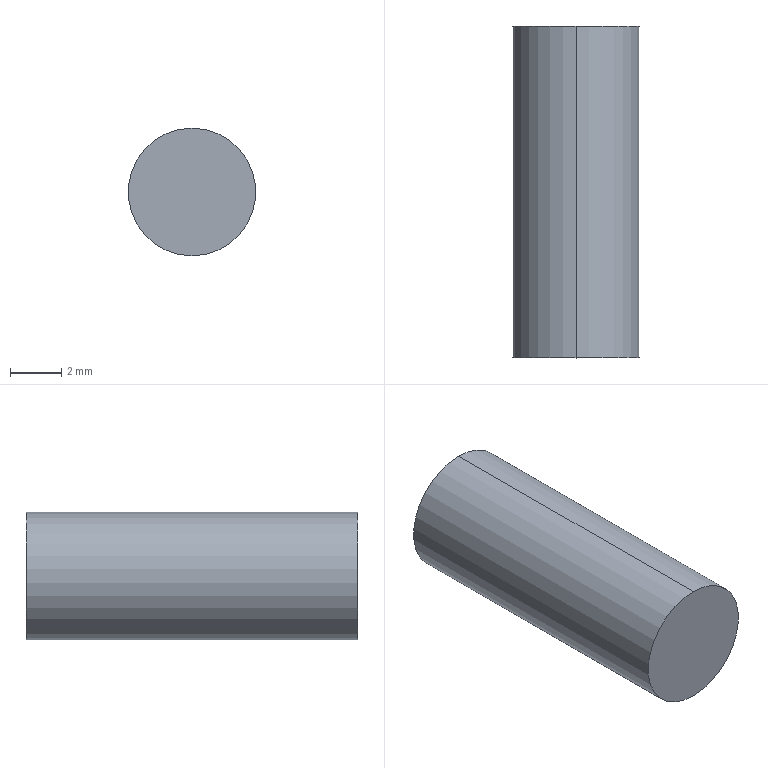Part | SolidWorks | features BaseBody 1 | 1 solid | 4 faces | box 5 x 13 x 5 mm | volume 255.254 mm3 | cylinder 2 | plane 2 | commonest cylinder face diameters 5 x2
STEP:
#1=CARTESIAN_POINT('',(-129.54,300.,170.282));
#2=VERTEX_POINT('',#1);
#3=CARTESIAN_POINT('',(-129.54,300.,175.282));
#4=VERTEX_POINT('',#3);
#5=CARTESIAN_POINT('',(-129.54,300.,172.782));
#6=DIRECTION('',(0.,-1.,0.));
#7=DIRECTION('',(1.,0.,0.));
#8=AXIS2_PLACEMENT_3D('',#5,#6,#7);
#9=CIRCLE('',#8,2.5);
#10=EDGE_CURVE('',#2,#4,#9,.T.);
#11=ORIENTED_EDGE('',*,*,#10,.T.);
#12=CARTESIAN_POINT('',(-129.54,287.,175.282));
#13=VERTEX_POINT('',#12);
#14=CARTESIAN_POINT('',(-129.54,300.,175.282));
#15=DIRECTION('',(0.,-1.,0.));
#16=VECTOR('',#15,1000.);
#17=LINE('',#14,#16);
#18=EDGE_CURVE('',#4,#13,#17,.T.);
#19=ORIENTED_EDGE('',*,*,#18,.T.);
#20=CARTESIAN_POINT('',(-129.54,287.,170.282));
#21=VERTEX_POINT('',#20);
#22=CARTESIAN_POINT('',(-129.54,287.,172.782));
#23=DIRECTION('',(0.,-1.,0.));
#24=DIRECTION('',(1.,0.,0.));
#25=AXIS2_PLACEMENT_3D('',#22,#23,#24);
#26=CIRCLE('',#25,2.5);
#27=EDGE_CURVE('',#21,#13,#26,.T.);
#28=ORIENTED_EDGE('',*,*,#27,.F.);
#29=CARTESIAN_POINT('',(-129.54,300.,170.282));
#30=DIRECTION('',(0.,-1.,0.));
#31=VECTOR('',#30,1000.);
#32=LINE('',#29,#31);
#33=EDGE_CURVE('',#2,#21,#32,.T.);
#34=ORIENTED_EDGE('',*,*,#33,.F.);
#35=EDGE_LOOP('',(#11,#19,#28,#34));
#36=FACE_OUTER_BOUND('',#35,.T.);
#37=CARTESIAN_POINT('',(-129.54,300.,172.782));
#38=DIRECTION('',(0.,-1.,0.));
#39=DIRECTION('',(0.,0.,-1.));
#40=AXIS2_PLACEMENT_3D('',#37,#38,#39);
#41=CYLINDRICAL_SURFACE('',#40,2.5);
#42=ADVANCED_FACE('',(#36),#41,.T.);
#43=ORIENTED_EDGE('',*,*,#18,.F.);
#44=CARTESIAN_POINT('',(-129.54,300.,172.782));
#45=DIRECTION('',(0.,-1.,0.));
#46=DIRECTION('',(1.,0.,0.));
#47=AXIS2_PLACEMENT_3D('',#44,#45,#46);
#48=CIRCLE('',#47,2.5);
#49=EDGE_CURVE('',#4,#2,#48,.T.);
#50=ORIENTED_EDGE('',*,*,#49,.T.);
#51=ORIENTED_EDGE('',*,*,#33,.T.);
#52=CARTESIAN_POINT('',(-129.54,287.,172.782));
#53=DIRECTION('',(0.,-1.,0.));
#54=DIRECTION('',(1.,0.,0.));
#55=AXIS2_PLACEMENT_3D('',#52,#53,#54);
#56=CIRCLE('',#55,2.5);
#57=EDGE_CURVE('',#13,#21,#56,.T.);
#58=ORIENTED_EDGE('',*,*,#57,.F.);
#59=EDGE_LOOP('',(#43,#50,#51,#58));
#60=FACE_OUTER_BOUND('',#59,.T.);
#61=CARTESIAN_POINT('',(-129.54,300.,172.782));
#62=DIRECTION('',(0.,-1.,0.));
#63=DIRECTION('',(0.,0.,-1.));
#64=AXIS2_PLACEMENT_3D('',#61,#62,#63);
#65=CYLINDRICAL_SURFACE('',#64,2.5);
#66=ADVANCED_FACE('',(#60),#65,.T.);
#67=ORIENTED_EDGE('',*,*,#10,.F.);
#68=ORIENTED_EDGE('',*,*,#49,.F.);
#69=EDGE_LOOP('',(#67,#68));
#70=FACE_OUTER_BOUND('',#69,.T.);
#71=CARTESIAN_POINT('',(-129.54,300.,172.782));
#72=DIRECTION('',(0.,-1.,0.));
#73=DIRECTION('',(0.,0.,-1.));
#74=AXIS2_PLACEMENT_3D('',#71,#72,#73);
#75=PLANE('',#74);
#76=ADVANCED_FACE('',(#70),#75,.F.);
#77=ORIENTED_EDGE('',*,*,#27,.T.);
#78=ORIENTED_EDGE('',*,*,#57,.T.);
#79=EDGE_LOOP('',(#77,#78));
#80=FACE_OUTER_BOUND('',#79,.T.);
#81=CARTESIAN_POINT('',(-129.54,287.,172.782));
#82=DIRECTION('',(0.,-1.,0.));
#83=DIRECTION('',(0.,0.,-1.));
#84=AXIS2_PLACEMENT_3D('',#81,#82,#83);
#85=PLANE('',#84);
#86=ADVANCED_FACE('',(#80),#85,.T.);
#87=CLOSED_SHELL('',(#42,#66,#76,#86));
#88=MANIFOLD_SOLID_BREP('',#87);
#89=CARTESIAN_POINT('',(0.,0.,0.));
#90=DIRECTION('',(0.,0.,1.));
#91=DIRECTION('',(1.,0.,0.));
#92=AXIS2_PLACEMENT_3D('',#89,#90,#91);
#93=(LENGTH_UNIT()NAMED_UNIT(*)SI_UNIT(.MILLI.,.METRE.));
#94=UNCERTAINTY_MEASURE_WITH_UNIT(LENGTH_MEASURE(0.00001),#93,'','');
#95=(NAMED_UNIT(*)PLANE_ANGLE_UNIT()SI_UNIT($,.RADIAN.));
#96=(NAMED_UNIT(*)SI_UNIT($,.STERADIAN.)SOLID_ANGLE_UNIT());
#97=(GEOMETRIC_REPRESENTATION_CONTEXT(3)GLOBAL_UNCERTAINTY_ASSIGNED_CONTEXT((#94))GLOBAL_UNIT_ASSIGNED_CONTEXT((#93,#95,#96))REPRESENTATION_CONTEXT('',''));
#98=ADVANCED_BREP_SHAPE_REPRESENTATION('',(#88,#92),#97);